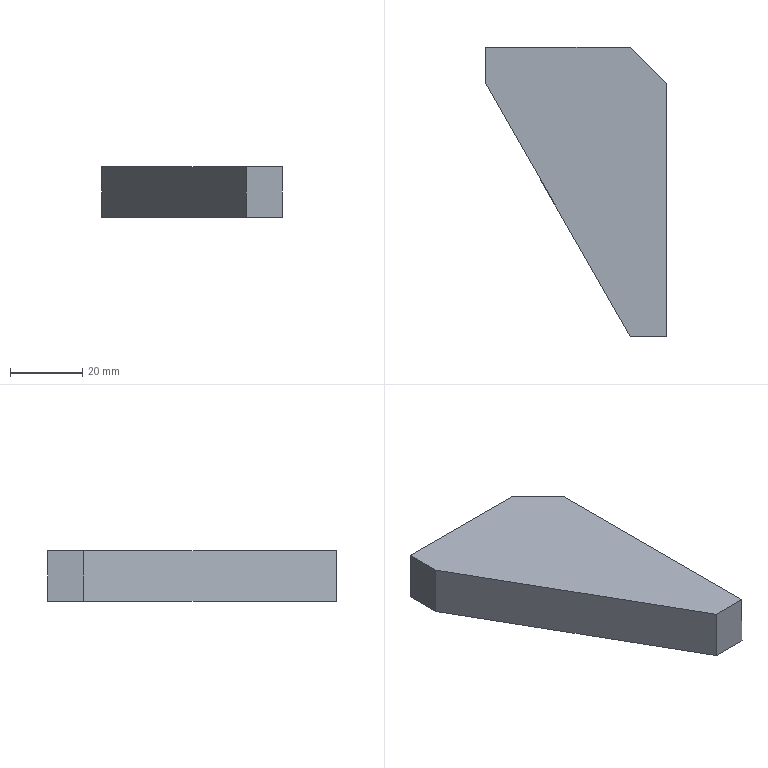Part | SolidWorks | features Chamfer 1, Extrusion 1 | 1 solid | 8 faces | box 50 x 80 x 14 mm | volume 35700 mm3 | plane 8
STEP:
#1=CARTESIAN_POINT('',(-50.,0.,0.));
#2=VERTEX_POINT('',#1);
#3=CARTESIAN_POINT('',(-10.,0.,0.));
#4=VERTEX_POINT('',#3);
#5=CARTESIAN_POINT('',(-50.,0.,0.));
#6=DIRECTION('',(1.,0.,0.));
#7=VECTOR('',#6,1000.);
#8=LINE('',#5,#7);
#9=EDGE_CURVE('',#2,#4,#8,.T.);
#10=ORIENTED_EDGE('',*,*,#9,.T.);
#11=CARTESIAN_POINT('',(-10.,0.,-14.));
#12=VERTEX_POINT('',#11);
#13=CARTESIAN_POINT('',(-10.,0.,-14.));
#14=DIRECTION('',(0.,0.,-1.));
#15=VECTOR('',#14,1000.);
#16=LINE('',#13,#15);
#17=EDGE_CURVE('',#4,#12,#16,.T.);
#18=ORIENTED_EDGE('',*,*,#17,.T.);
#19=CARTESIAN_POINT('',(-50.,0.,-14.));
#20=VERTEX_POINT('',#19);
#21=CARTESIAN_POINT('',(-50.,0.,-14.));
#22=DIRECTION('',(1.,0.,0.));
#23=VECTOR('',#22,1000.);
#24=LINE('',#21,#23);
#25=EDGE_CURVE('',#20,#12,#24,.T.);
#26=ORIENTED_EDGE('',*,*,#25,.F.);
#27=CARTESIAN_POINT('',(-50.,0.,-14.));
#28=DIRECTION('',(0.,0.,1.));
#29=VECTOR('',#28,1000.);
#30=LINE('',#27,#29);
#31=EDGE_CURVE('',#20,#2,#30,.T.);
#32=ORIENTED_EDGE('',*,*,#31,.T.);
#33=EDGE_LOOP('',(#10,#18,#26,#32));
#34=FACE_OUTER_BOUND('',#33,.T.);
#35=CARTESIAN_POINT('',(-50.,0.,-14.));
#36=DIRECTION('',(0.,-1.,0.));
#37=DIRECTION('',(0.,0.,-1.));
#38=AXIS2_PLACEMENT_3D('',#35,#36,#37);
#39=PLANE('',#38);
#40=ADVANCED_FACE('',(#34),#39,.F.);
#41=CARTESIAN_POINT('',(0.,-10.,-14.));
#42=VERTEX_POINT('',#41);
#43=CARTESIAN_POINT('',(0.,-80.,-14.));
#44=VERTEX_POINT('',#43);
#45=CARTESIAN_POINT('',(0.,0.,-14.));
#46=DIRECTION('',(0.,-1.,0.));
#47=VECTOR('',#46,1000.);
#48=LINE('',#45,#47);
#49=EDGE_CURVE('',#42,#44,#48,.T.);
#50=ORIENTED_EDGE('',*,*,#49,.F.);
#51=CARTESIAN_POINT('',(0.,-10.,0.));
#52=VERTEX_POINT('',#51);
#53=CARTESIAN_POINT('',(0.,-10.,-14.));
#54=DIRECTION('',(0.,0.,1.));
#55=VECTOR('',#54,1000.);
#56=LINE('',#53,#55);
#57=EDGE_CURVE('',#42,#52,#56,.T.);
#58=ORIENTED_EDGE('',*,*,#57,.T.);
#59=CARTESIAN_POINT('',(0.,-80.,0.));
#60=VERTEX_POINT('',#59);
#61=CARTESIAN_POINT('',(0.,0.,0.));
#62=DIRECTION('',(0.,-1.,0.));
#63=VECTOR('',#62,1000.);
#64=LINE('',#61,#63);
#65=EDGE_CURVE('',#52,#60,#64,.T.);
#66=ORIENTED_EDGE('',*,*,#65,.T.);
#67=CARTESIAN_POINT('',(0.,-80.,-14.));
#68=DIRECTION('',(0.,0.,1.));
#69=VECTOR('',#68,1000.);
#70=LINE('',#67,#69);
#71=EDGE_CURVE('',#44,#60,#70,.T.);
#72=ORIENTED_EDGE('',*,*,#71,.F.);
#73=EDGE_LOOP('',(#50,#58,#66,#72));
#74=FACE_OUTER_BOUND('',#73,.T.);
#75=CARTESIAN_POINT('',(0.,0.,-14.));
#76=DIRECTION('',(-1.,0.,0.));
#77=DIRECTION('',(0.,0.,1.));
#78=AXIS2_PLACEMENT_3D('',#75,#76,#77);
#79=PLANE('',#78);
#80=ADVANCED_FACE('',(#74),#79,.F.);
#81=CARTESIAN_POINT('',(-10.,-80.,0.));
#82=VERTEX_POINT('',#81);
#83=CARTESIAN_POINT('',(0.,-80.,0.));
#84=DIRECTION('',(-1.,0.,0.));
#85=VECTOR('',#84,1000.);
#86=LINE('',#83,#85);
#87=EDGE_CURVE('',#60,#82,#86,.T.);
#88=ORIENTED_EDGE('',*,*,#87,.T.);
#89=CARTESIAN_POINT('',(-10.,-80.,-14.));
#90=VERTEX_POINT('',#89);
#91=CARTESIAN_POINT('',(-10.,-80.,-14.));
#92=DIRECTION('',(0.,0.,1.));
#93=VECTOR('',#92,1000.);
#94=LINE('',#91,#93);
#95=EDGE_CURVE('',#90,#82,#94,.T.);
#96=ORIENTED_EDGE('',*,*,#95,.F.);
#97=CARTESIAN_POINT('',(0.,-80.,-14.));
#98=DIRECTION('',(-1.,0.,0.));
#99=VECTOR('',#98,1000.);
#100=LINE('',#97,#99);
#101=EDGE_CURVE('',#44,#90,#100,.T.);
#102=ORIENTED_EDGE('',*,*,#101,.F.);
#103=ORIENTED_EDGE('',*,*,#71,.T.);
#104=EDGE_LOOP('',(#88,#96,#102,#103));
#105=FACE_OUTER_BOUND('',#104,.T.);
#106=CARTESIAN_POINT('',(0.,-80.,-14.));
#107=DIRECTION('',(0.,1.,0.));
#108=DIRECTION('',(0.,0.,1.));
#109=AXIS2_PLACEMENT_3D('',#106,#107,#108);
#110=PLANE('',#109);
#111=ADVANCED_FACE('',(#105),#110,.F.);
#112=CARTESIAN_POINT('',(-50.,-10.,0.));
#113=VERTEX_POINT('',#112);
#114=CARTESIAN_POINT('',(-10.,-80.,0.));
#115=DIRECTION('',(-0.4961,0.8682,0.));
#116=VECTOR('',#115,1000.);
#117=LINE('',#114,#116);
#118=EDGE_CURVE('',#82,#113,#117,.T.);
#119=ORIENTED_EDGE('',*,*,#118,.T.);
#120=CARTESIAN_POINT('',(-50.,-10.,-14.));
#121=VERTEX_POINT('',#120);
#122=CARTESIAN_POINT('',(-50.,-10.,-14.));
#123=DIRECTION('',(0.,0.,1.));
#124=VECTOR('',#123,1000.);
#125=LINE('',#122,#124);
#126=EDGE_CURVE('',#121,#113,#125,.T.);
#127=ORIENTED_EDGE('',*,*,#126,.F.);
#128=CARTESIAN_POINT('',(-10.,-80.,-14.));
#129=DIRECTION('',(-0.4961,0.8682,0.));
#130=VECTOR('',#129,1000.);
#131=LINE('',#128,#130);
#132=EDGE_CURVE('',#90,#121,#131,.T.);
#133=ORIENTED_EDGE('',*,*,#132,.F.);
#134=ORIENTED_EDGE('',*,*,#95,.T.);
#135=EDGE_LOOP('',(#119,#127,#133,#134));
#136=FACE_OUTER_BOUND('',#135,.T.);
#137=CARTESIAN_POINT('',(-10.,-80.,-14.));
#138=DIRECTION('',(0.8682,0.4961,0.));
#139=DIRECTION('',(-0.4961,0.8682,0.));
#140=AXIS2_PLACEMENT_3D('',#137,#138,#139);
#141=PLANE('',#140);
#142=ADVANCED_FACE('',(#136),#141,.F.);
#143=CARTESIAN_POINT('',(-50.,-10.,0.));
#144=DIRECTION('',(0.,1.,0.));
#145=VECTOR('',#144,1000.);
#146=LINE('',#143,#145);
#147=EDGE_CURVE('',#113,#2,#146,.T.);
#148=ORIENTED_EDGE('',*,*,#147,.T.);
#149=ORIENTED_EDGE('',*,*,#31,.F.);
#150=CARTESIAN_POINT('',(-50.,-10.,-14.));
#151=DIRECTION('',(0.,1.,0.));
#152=VECTOR('',#151,1000.);
#153=LINE('',#150,#152);
#154=EDGE_CURVE('',#121,#20,#153,.T.);
#155=ORIENTED_EDGE('',*,*,#154,.F.);
#156=ORIENTED_EDGE('',*,*,#126,.T.);
#157=EDGE_LOOP('',(#148,#149,#155,#156));
#158=FACE_OUTER_BOUND('',#157,.T.);
#159=CARTESIAN_POINT('',(-50.,-10.,-14.));
#160=DIRECTION('',(1.,0.,0.));
#161=DIRECTION('',(0.,1.,0.));
#162=AXIS2_PLACEMENT_3D('',#159,#160,#161);
#163=PLANE('',#162);
#164=ADVANCED_FACE('',(#158),#163,.F.);
#165=ORIENTED_EDGE('',*,*,#25,.T.);
#166=CARTESIAN_POINT('',(-5.,-5.,-14.));
#167=DIRECTION('',(0.7071,-0.7071,0.));
#168=VECTOR('',#167,1000.);
#169=LINE('',#166,#168);
#170=EDGE_CURVE('',#12,#42,#169,.T.);
#171=ORIENTED_EDGE('',*,*,#170,.T.);
#172=ORIENTED_EDGE('',*,*,#49,.T.);
#173=ORIENTED_EDGE('',*,*,#101,.T.);
#174=ORIENTED_EDGE('',*,*,#132,.T.);
#175=ORIENTED_EDGE('',*,*,#154,.T.);
#176=EDGE_LOOP('',(#165,#171,#172,#173,#174,#175));
#177=FACE_OUTER_BOUND('',#176,.T.);
#178=CARTESIAN_POINT('',(0.,0.,-14.));
#179=DIRECTION('',(0.,0.,-1.));
#180=DIRECTION('',(-1.,0.,0.));
#181=AXIS2_PLACEMENT_3D('',#178,#179,#180);
#182=PLANE('',#181);
#183=ADVANCED_FACE('',(#177),#182,.T.);
#184=ORIENTED_EDGE('',*,*,#65,.F.);
#185=CARTESIAN_POINT('',(0.,-10.,0.));
#186=DIRECTION('',(-0.7071,0.7071,0.));
#187=VECTOR('',#186,1000.);
#188=LINE('',#185,#187);
#189=EDGE_CURVE('',#52,#4,#188,.T.);
#190=ORIENTED_EDGE('',*,*,#189,.T.);
#191=ORIENTED_EDGE('',*,*,#9,.F.);
#192=ORIENTED_EDGE('',*,*,#147,.F.);
#193=ORIENTED_EDGE('',*,*,#118,.F.);
#194=ORIENTED_EDGE('',*,*,#87,.F.);
#195=EDGE_LOOP('',(#184,#190,#191,#192,#193,#194));
#196=FACE_OUTER_BOUND('',#195,.T.);
#197=CARTESIAN_POINT('',(0.,0.,0.));
#198=DIRECTION('',(0.,0.,-1.));
#199=DIRECTION('',(-1.,0.,0.));
#200=AXIS2_PLACEMENT_3D('',#197,#198,#199);
#201=PLANE('',#200);
#202=ADVANCED_FACE('',(#196),#201,.F.);
#203=ORIENTED_EDGE('',*,*,#170,.F.);
#204=ORIENTED_EDGE('',*,*,#17,.F.);
#205=ORIENTED_EDGE('',*,*,#189,.F.);
#206=ORIENTED_EDGE('',*,*,#57,.F.);
#207=EDGE_LOOP('',(#203,#204,#205,#206));
#208=FACE_OUTER_BOUND('',#207,.T.);
#209=CARTESIAN_POINT('',(0.,-10.,-14.));
#210=DIRECTION('',(-0.7071,-0.7071,0.));
#211=DIRECTION('',(0.,0.,1.));
#212=AXIS2_PLACEMENT_3D('',#209,#210,#211);
#213=PLANE('',#212);
#214=ADVANCED_FACE('',(#208),#213,.F.);
#215=CLOSED_SHELL('',(#40,#80,#111,#142,#164,#183,#202,#214));
#216=MANIFOLD_SOLID_BREP('',#215);
#217=CARTESIAN_POINT('',(0.,0.,0.));
#218=DIRECTION('',(0.,0.,1.));
#219=DIRECTION('',(1.,0.,0.));
#220=AXIS2_PLACEMENT_3D('',#217,#218,#219);
#221=(LENGTH_UNIT()NAMED_UNIT(*)SI_UNIT(.MILLI.,.METRE.));
#222=UNCERTAINTY_MEASURE_WITH_UNIT(LENGTH_MEASURE(0.00001),#221,'','');
#223=(NAMED_UNIT(*)PLANE_ANGLE_UNIT()SI_UNIT($,.RADIAN.));
#224=(NAMED_UNIT(*)SI_UNIT($,.STERADIAN.)SOLID_ANGLE_UNIT());
#225=(GEOMETRIC_REPRESENTATION_CONTEXT(3)GLOBAL_UNCERTAINTY_ASSIGNED_CONTEXT((#222))GLOBAL_UNIT_ASSIGNED_CONTEXT((#221,#223,#224))REPRESENTATION_CONTEXT('',''));
#226=ADVANCED_BREP_SHAPE_REPRESENTATION('',(#216,#220),#225);